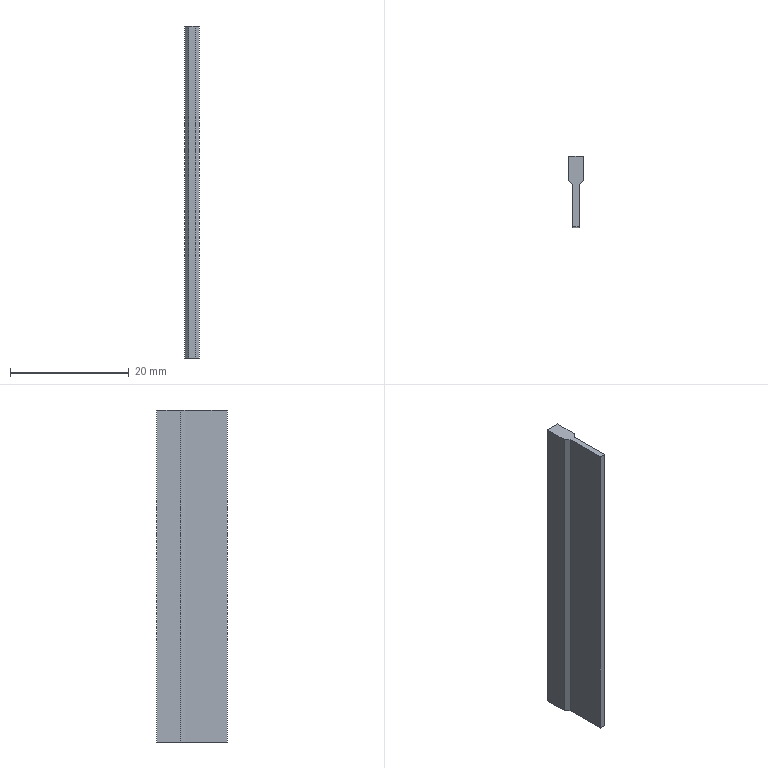Part | NX | features BREP 2 | 2 solids | 20 faces | box 2.42 x 11.896 x 56 mm | volume 2041 mm3 | plane 20
STEP:
#1=CARTESIAN_POINT('',(-0.5101,1.23,-4.));
#2=VERTEX_POINT('',#1);
#3=CARTESIAN_POINT('',(-0.5101,1.23,52.));
#4=VERTEX_POINT('',#3);
#5=CARTESIAN_POINT('',(-0.5101,1.23,0.));
#6=DIRECTION('',(0.,0.,1.));
#7=VECTOR('',#6,1000.);
#8=LINE('',#5,#7);
#9=EDGE_CURVE('',#2,#4,#8,.T.);
#10=ORIENTED_EDGE('',*,*,#9,.T.);
#11=CARTESIAN_POINT('',(-1.21,1.93,52.));
#12=VERTEX_POINT('',#11);
#13=CARTESIAN_POINT('',(-0.5101,1.23,52.));
#14=DIRECTION('',(0.7071,-0.7071,0.));
#15=VECTOR('',#14,1000.);
#16=LINE('',#13,#15);
#17=EDGE_CURVE('',#12,#4,#16,.T.);
#18=ORIENTED_EDGE('',*,*,#17,.F.);
#19=CARTESIAN_POINT('',(-1.21,1.93,-4.));
#20=VERTEX_POINT('',#19);
#21=CARTESIAN_POINT('',(-1.21,1.93,0.));
#22=DIRECTION('',(0.,0.,1.));
#23=VECTOR('',#22,1000.);
#24=LINE('',#21,#23);
#25=EDGE_CURVE('',#20,#12,#24,.T.);
#26=ORIENTED_EDGE('',*,*,#25,.F.);
#27=CARTESIAN_POINT('',(-0.5101,1.23,-4.));
#28=DIRECTION('',(0.7071,-0.7071,0.));
#29=VECTOR('',#28,1000.);
#30=LINE('',#27,#29);
#31=EDGE_CURVE('',#20,#2,#30,.T.);
#32=ORIENTED_EDGE('',*,*,#31,.T.);
#33=EDGE_LOOP('',(#10,#18,#26,#32));
#34=FACE_BOUND('',#33,.T.);
#35=CARTESIAN_POINT('',(-0.5101,1.23,0.));
#36=DIRECTION('',(0.7071,0.7071,0.));
#37=DIRECTION('',(0.7071,-0.7071,0.));
#38=AXIS2_PLACEMENT_3D('',#35,#36,#37);
#39=PLANE('',#38);
#40=ADVANCED_FACE('',(#34),#39,.F.);
#41=ORIENTED_EDGE('',*,*,#25,.T.);
#42=CARTESIAN_POINT('',(-1.21,5.923,52.));
#43=VERTEX_POINT('',#42);
#44=CARTESIAN_POINT('',(-1.21,-19.679,52.));
#45=DIRECTION('',(0.,-1.,0.));
#46=VECTOR('',#45,1000.);
#47=LINE('',#44,#46);
#48=EDGE_CURVE('',#43,#12,#47,.T.);
#49=ORIENTED_EDGE('',*,*,#48,.F.);
#50=CARTESIAN_POINT('',(-1.21,5.923,-4.));
#51=VERTEX_POINT('',#50);
#52=CARTESIAN_POINT('',(-1.21,5.923,0.));
#53=DIRECTION('',(0.,0.,1.));
#54=VECTOR('',#53,1000.);
#55=LINE('',#52,#54);
#56=EDGE_CURVE('',#51,#43,#55,.T.);
#57=ORIENTED_EDGE('',*,*,#56,.F.);
#58=CARTESIAN_POINT('',(-1.21,-19.679,-4.));
#59=DIRECTION('',(0.,-1.,0.));
#60=VECTOR('',#59,1000.);
#61=LINE('',#58,#60);
#62=EDGE_CURVE('',#51,#20,#61,.T.);
#63=ORIENTED_EDGE('',*,*,#62,.T.);
#64=EDGE_LOOP('',(#41,#49,#57,#63));
#65=FACE_BOUND('',#64,.T.);
#66=CARTESIAN_POINT('',(-1.21,1.93,0.));
#67=DIRECTION('',(1.,0.,0.));
#68=DIRECTION('',(0.,-1.,0.));
#69=AXIS2_PLACEMENT_3D('',#66,#67,#68);
#70=PLANE('',#69);
#71=ADVANCED_FACE('',(#65),#70,.F.);
#72=ORIENTED_EDGE('',*,*,#56,.T.);
#73=CARTESIAN_POINT('',(1.21,5.923,52.));
#74=VERTEX_POINT('',#73);
#75=CARTESIAN_POINT('',(-10.54,5.923,52.));
#76=DIRECTION('',(-1.,0.,0.));
#77=VECTOR('',#76,1000.);
#78=LINE('',#75,#77);
#79=EDGE_CURVE('',#74,#43,#78,.T.);
#80=ORIENTED_EDGE('',*,*,#79,.F.);
#81=CARTESIAN_POINT('',(1.21,5.923,-4.));
#82=VERTEX_POINT('',#81);
#83=CARTESIAN_POINT('',(1.21,5.923,0.));
#84=DIRECTION('',(0.,0.,1.));
#85=VECTOR('',#84,1000.);
#86=LINE('',#83,#85);
#87=EDGE_CURVE('',#82,#74,#86,.T.);
#88=ORIENTED_EDGE('',*,*,#87,.F.);
#89=CARTESIAN_POINT('',(-10.54,5.923,-4.));
#90=DIRECTION('',(-1.,0.,0.));
#91=VECTOR('',#90,1000.);
#92=LINE('',#89,#91);
#93=EDGE_CURVE('',#82,#51,#92,.T.);
#94=ORIENTED_EDGE('',*,*,#93,.T.);
#95=EDGE_LOOP('',(#72,#80,#88,#94));
#96=FACE_BOUND('',#95,.T.);
#97=CARTESIAN_POINT('',(-10.54,5.923,0.));
#98=DIRECTION('',(0.,1.,0.));
#99=DIRECTION('',(1.,0.,0.));
#100=AXIS2_PLACEMENT_3D('',#97,#98,#99);
#101=PLANE('',#100);
#102=ADVANCED_FACE('',(#96),#101,.T.);
#103=ORIENTED_EDGE('',*,*,#87,.T.);
#104=CARTESIAN_POINT('',(1.21,1.923,52.));
#105=VERTEX_POINT('',#104);
#106=CARTESIAN_POINT('',(1.21,-19.679,52.));
#107=DIRECTION('',(0.,1.,0.));
#108=VECTOR('',#107,1000.);
#109=LINE('',#106,#108);
#110=EDGE_CURVE('',#105,#74,#109,.T.);
#111=ORIENTED_EDGE('',*,*,#110,.F.);
#112=CARTESIAN_POINT('',(1.21,1.923,-4.));
#113=VERTEX_POINT('',#112);
#114=CARTESIAN_POINT('',(1.21,1.923,0.));
#115=DIRECTION('',(0.,0.,1.));
#116=VECTOR('',#115,1000.);
#117=LINE('',#114,#116);
#118=EDGE_CURVE('',#113,#105,#117,.T.);
#119=ORIENTED_EDGE('',*,*,#118,.F.);
#120=CARTESIAN_POINT('',(1.21,-19.679,-4.));
#121=DIRECTION('',(0.,1.,0.));
#122=VECTOR('',#121,1000.);
#123=LINE('',#120,#122);
#124=EDGE_CURVE('',#113,#82,#123,.T.);
#125=ORIENTED_EDGE('',*,*,#124,.T.);
#126=EDGE_LOOP('',(#103,#111,#119,#125));
#127=FACE_BOUND('',#126,.T.);
#128=CARTESIAN_POINT('',(1.21,5.923,0.));
#129=DIRECTION('',(-1.,0.,0.));
#130=DIRECTION('',(0.,1.,0.));
#131=AXIS2_PLACEMENT_3D('',#128,#129,#130);
#132=PLANE('',#131);
#133=ADVANCED_FACE('',(#127),#132,.F.);
#134=ORIENTED_EDGE('',*,*,#118,.T.);
#135=CARTESIAN_POINT('',(0.5101,1.223,52.));
#136=VERTEX_POINT('',#135);
#137=CARTESIAN_POINT('',(1.21,1.923,52.));
#138=DIRECTION('',(0.7071,0.7071,0.));
#139=VECTOR('',#138,1000.);
#140=LINE('',#137,#139);
#141=EDGE_CURVE('',#136,#105,#140,.T.);
#142=ORIENTED_EDGE('',*,*,#141,.F.);
#143=CARTESIAN_POINT('',(0.5101,1.223,-4.));
#144=VERTEX_POINT('',#143);
#145=CARTESIAN_POINT('',(0.5101,1.223,0.));
#146=DIRECTION('',(0.,0.,1.));
#147=VECTOR('',#146,1000.);
#148=LINE('',#145,#147);
#149=EDGE_CURVE('',#144,#136,#148,.T.);
#150=ORIENTED_EDGE('',*,*,#149,.F.);
#151=CARTESIAN_POINT('',(1.21,1.923,-4.));
#152=DIRECTION('',(0.7071,0.7071,0.));
#153=VECTOR('',#152,1000.);
#154=LINE('',#151,#153);
#155=EDGE_CURVE('',#144,#113,#154,.T.);
#156=ORIENTED_EDGE('',*,*,#155,.T.);
#157=EDGE_LOOP('',(#134,#142,#150,#156));
#158=FACE_BOUND('',#157,.T.);
#159=CARTESIAN_POINT('',(1.21,1.923,0.));
#160=DIRECTION('',(-0.7071,0.7071,0.));
#161=DIRECTION('',(0.7071,0.7071,0.));
#162=AXIS2_PLACEMENT_3D('',#159,#160,#161);
#163=PLANE('',#162);
#164=ADVANCED_FACE('',(#158),#163,.F.);
#165=CARTESIAN_POINT('',(0.5101,-5.973,-4.));
#166=VERTEX_POINT('',#165);
#167=CARTESIAN_POINT('',(0.5101,-5.973,52.));
#168=VERTEX_POINT('',#167);
#169=CARTESIAN_POINT('',(0.5101,-5.973,0.));
#170=DIRECTION('',(0.,0.,1.));
#171=VECTOR('',#170,1000.);
#172=LINE('',#169,#171);
#173=EDGE_CURVE('',#166,#168,#172,.T.);
#174=ORIENTED_EDGE('',*,*,#173,.F.);
#175=CARTESIAN_POINT('',(0.5101,-19.679,-4.));
#176=DIRECTION('',(0.,1.,0.));
#177=VECTOR('',#176,1000.);
#178=LINE('',#175,#177);
#179=EDGE_CURVE('',#166,#144,#178,.T.);
#180=ORIENTED_EDGE('',*,*,#179,.T.);
#181=ORIENTED_EDGE('',*,*,#149,.T.);
#182=CARTESIAN_POINT('',(0.5101,-19.679,52.));
#183=DIRECTION('',(0.,1.,0.));
#184=VECTOR('',#183,1000.);
#185=LINE('',#182,#184);
#186=EDGE_CURVE('',#168,#136,#185,.T.);
#187=ORIENTED_EDGE('',*,*,#186,.F.);
#188=EDGE_LOOP('',(#174,#180,#181,#187));
#189=FACE_BOUND('',#188,.T.);
#190=CARTESIAN_POINT('',(0.5101,-5.28,0.));
#191=DIRECTION('',(-1.,0.,0.));
#192=DIRECTION('',(0.,1.,0.));
#193=AXIS2_PLACEMENT_3D('',#190,#191,#192);
#194=PLANE('',#193);
#195=ADVANCED_FACE('',(#189),#194,.F.);
#196=ORIENTED_EDGE('',*,*,#173,.T.);
#197=CARTESIAN_POINT('',(-0.5101,-5.973,52.));
#198=VERTEX_POINT('',#197);
#199=CARTESIAN_POINT('',(-10.54,-5.973,52.));
#200=DIRECTION('',(1.,0.,0.));
#201=VECTOR('',#200,1000.);
#202=LINE('',#199,#201);
#203=EDGE_CURVE('',#198,#168,#202,.T.);
#204=ORIENTED_EDGE('',*,*,#203,.F.);
#205=CARTESIAN_POINT('',(-0.5101,-5.973,-4.));
#206=VERTEX_POINT('',#205);
#207=CARTESIAN_POINT('',(-0.5101,-5.973,0.));
#208=DIRECTION('',(0.,0.,1.));
#209=VECTOR('',#208,1000.);
#210=LINE('',#207,#209);
#211=EDGE_CURVE('',#206,#198,#210,.T.);
#212=ORIENTED_EDGE('',*,*,#211,.F.);
#213=CARTESIAN_POINT('',(-10.54,-5.973,-4.));
#214=DIRECTION('',(1.,0.,0.));
#215=VECTOR('',#214,1000.);
#216=LINE('',#213,#215);
#217=EDGE_CURVE('',#206,#166,#216,.T.);
#218=ORIENTED_EDGE('',*,*,#217,.T.);
#219=EDGE_LOOP('',(#196,#204,#212,#218));
#220=FACE_BOUND('',#219,.T.);
#221=CARTESIAN_POINT('',(-10.54,-5.973,0.));
#222=DIRECTION('',(0.,-1.,0.));
#223=DIRECTION('',(-1.,0.,0.));
#224=AXIS2_PLACEMENT_3D('',#221,#222,#223);
#225=PLANE('',#224);
#226=ADVANCED_FACE('',(#220),#225,.T.);
#227=CARTESIAN_POINT('',(-0.5101,-19.679,-4.));
#228=DIRECTION('',(0.,-1.,0.));
#229=VECTOR('',#228,1000.);
#230=LINE('',#227,#229);
#231=EDGE_CURVE('',#2,#206,#230,.T.);
#232=ORIENTED_EDGE('',*,*,#231,.T.);
#233=ORIENTED_EDGE('',*,*,#211,.T.);
#234=CARTESIAN_POINT('',(-0.5101,-19.679,52.));
#235=DIRECTION('',(0.,-1.,0.));
#236=VECTOR('',#235,1000.);
#237=LINE('',#234,#236);
#238=EDGE_CURVE('',#4,#198,#237,.T.);
#239=ORIENTED_EDGE('',*,*,#238,.F.);
#240=ORIENTED_EDGE('',*,*,#9,.F.);
#241=EDGE_LOOP('',(#232,#233,#239,#240));
#242=FACE_BOUND('',#241,.T.);
#243=CARTESIAN_POINT('',(-0.5101,-5.28,0.));
#244=DIRECTION('',(1.,0.,0.));
#245=DIRECTION('',(0.,-1.,0.));
#246=AXIS2_PLACEMENT_3D('',#243,#244,#245);
#247=PLANE('',#246);
#248=ADVANCED_FACE('',(#242),#247,.F.);
#249=ORIENTED_EDGE('',*,*,#238,.T.);
#250=ORIENTED_EDGE('',*,*,#203,.T.);
#251=ORIENTED_EDGE('',*,*,#186,.T.);
#252=ORIENTED_EDGE('',*,*,#141,.T.);
#253=ORIENTED_EDGE('',*,*,#110,.T.);
#254=ORIENTED_EDGE('',*,*,#79,.T.);
#255=ORIENTED_EDGE('',*,*,#48,.T.);
#256=ORIENTED_EDGE('',*,*,#17,.T.);
#257=EDGE_LOOP('',(#249,#250,#251,#252,#253,#254,#255,#256));
#258=FACE_BOUND('',#257,.T.);
#259=CARTESIAN_POINT('',(-10.54,-19.679,52.));
#260=DIRECTION('',(0.,0.,1.));
#261=DIRECTION('',(-1.,0.,0.));
#262=AXIS2_PLACEMENT_3D('',#259,#260,#261);
#263=PLANE('',#262);
#264=ADVANCED_FACE('',(#258),#263,.T.);
#265=ORIENTED_EDGE('',*,*,#217,.F.);
#266=ORIENTED_EDGE('',*,*,#231,.F.);
#267=ORIENTED_EDGE('',*,*,#31,.F.);
#268=ORIENTED_EDGE('',*,*,#62,.F.);
#269=ORIENTED_EDGE('',*,*,#93,.F.);
#270=ORIENTED_EDGE('',*,*,#124,.F.);
#271=ORIENTED_EDGE('',*,*,#155,.F.);
#272=ORIENTED_EDGE('',*,*,#179,.F.);
#273=EDGE_LOOP('',(#265,#266,#267,#268,#269,#270,#271,#272));
#274=FACE_BOUND('',#273,.T.);
#275=CARTESIAN_POINT('',(-10.54,-19.679,-4.));
#276=DIRECTION('',(0.,0.,1.));
#277=DIRECTION('',(-1.,0.,0.));
#278=AXIS2_PLACEMENT_3D('',#275,#276,#277);
#279=PLANE('',#278);
#280=ADVANCED_FACE('',(#274),#279,.F.);
#281=CLOSED_SHELL('',(#40,#71,#102,#133,#164,#195,#226,#248,#264,#280));
#282=MANIFOLD_SOLID_BREP('',#281);
#283=CARTESIAN_POINT('',(-0.5101,1.23,-4.));
#284=VERTEX_POINT('',#283);
#285=CARTESIAN_POINT('',(-0.5101,1.23,52.));
#286=VERTEX_POINT('',#285);
#287=CARTESIAN_POINT('',(-0.5101,1.23,0.));
#288=DIRECTION('',(0.,0.,1.));
#289=VECTOR('',#288,1000.);
#290=LINE('',#287,#289);
#291=EDGE_CURVE('',#284,#286,#290,.T.);
#292=ORIENTED_EDGE('',*,*,#291,.T.);
#293=CARTESIAN_POINT('',(-1.21,1.93,52.));
#294=VERTEX_POINT('',#293);
#295=CARTESIAN_POINT('',(-0.5101,1.23,52.));
#296=DIRECTION('',(0.7071,-0.7071,0.));
#297=VECTOR('',#296,1000.);
#298=LINE('',#295,#297);
#299=EDGE_CURVE('',#294,#286,#298,.T.);
#300=ORIENTED_EDGE('',*,*,#299,.F.);
#301=CARTESIAN_POINT('',(-1.21,1.93,-4.));
#302=VERTEX_POINT('',#301);
#303=CARTESIAN_POINT('',(-1.21,1.93,0.));
#304=DIRECTION('',(0.,0.,1.));
#305=VECTOR('',#304,1000.);
#306=LINE('',#303,#305);
#307=EDGE_CURVE('',#302,#294,#306,.T.);
#308=ORIENTED_EDGE('',*,*,#307,.F.);
#309=CARTESIAN_POINT('',(-0.5101,1.23,-4.));
#310=DIRECTION('',(0.7071,-0.7071,0.));
#311=VECTOR('',#310,1000.);
#312=LINE('',#309,#311);
#313=EDGE_CURVE('',#302,#284,#312,.T.);
#314=ORIENTED_EDGE('',*,*,#313,.T.);
#315=EDGE_LOOP('',(#292,#300,#308,#314));
#316=FACE_BOUND('',#315,.T.);
#317=CARTESIAN_POINT('',(-0.5101,1.23,0.));
#318=DIRECTION('',(0.7071,0.7071,0.));
#319=DIRECTION('',(0.7071,-0.7071,0.));
#320=AXIS2_PLACEMENT_3D('',#317,#318,#319);
#321=PLANE('',#320);
#322=ADVANCED_FACE('',(#316),#321,.F.);
#323=ORIENTED_EDGE('',*,*,#307,.T.);
#324=CARTESIAN_POINT('',(-1.21,5.923,52.));
#325=VERTEX_POINT('',#324);
#326=CARTESIAN_POINT('',(-1.21,-19.679,52.));
#327=DIRECTION('',(0.,-1.,0.));
#328=VECTOR('',#327,1000.);
#329=LINE('',#326,#328);
#330=EDGE_CURVE('',#325,#294,#329,.T.);
#331=ORIENTED_EDGE('',*,*,#330,.F.);
#332=CARTESIAN_POINT('',(-1.21,5.923,-4.));
#333=VERTEX_POINT('',#332);
#334=CARTESIAN_POINT('',(-1.21,5.923,0.));
#335=DIRECTION('',(0.,0.,1.));
#336=VECTOR('',#335,1000.);
#337=LINE('',#334,#336);
#338=EDGE_CURVE('',#333,#325,#337,.T.);
#339=ORIENTED_EDGE('',*,*,#338,.F.);
#340=CARTESIAN_POINT('',(-1.21,-19.679,-4.));
#341=DIRECTION('',(0.,-1.,0.));
#342=VECTOR('',#341,1000.);
#343=LINE('',#340,#342);
#344=EDGE_CURVE('',#333,#302,#343,.T.);
#345=ORIENTED_EDGE('',*,*,#344,.T.);
#346=EDGE_LOOP('',(#323,#331,#339,#345));
#347=FACE_BOUND('',#346,.T.);
#348=CARTESIAN_POINT('',(-1.21,1.93,0.));
#349=DIRECTION('',(1.,0.,0.));
#350=DIRECTION('',(0.,-1.,0.));
#351=AXIS2_PLACEMENT_3D('',#348,#349,#350);
#352=PLANE('',#351);
#353=ADVANCED_FACE('',(#347),#352,.F.);
#354=ORIENTED_EDGE('',*,*,#338,.T.);
#355=CARTESIAN_POINT('',(1.21,5.923,52.));
#356=VERTEX_POINT('',#355);
#357=CARTESIAN_POINT('',(-10.54,5.923,52.));
#358=DIRECTION('',(-1.,0.,0.));
#359=VECTOR('',#358,1000.);
#360=LINE('',#357,#359);
#361=EDGE_CURVE('',#356,#325,#360,.T.);
#362=ORIENTED_EDGE('',*,*,#361,.F.);
#363=CARTESIAN_POINT('',(1.21,5.923,-4.));
#364=VERTEX_POINT('',#363);
#365=CARTESIAN_POINT('',(1.21,5.923,0.));
#366=DIRECTION('',(0.,0.,1.));
#367=VECTOR('',#366,1000.);
#368=LINE('',#365,#367);
#369=EDGE_CURVE('',#364,#356,#368,.T.);
#370=ORIENTED_EDGE('',*,*,#369,.F.);
#371=CARTESIAN_POINT('',(-10.54,5.923,-4.));
#372=DIRECTION('',(-1.,0.,0.));
#373=VECTOR('',#372,1000.);
#374=LINE('',#371,#373);
#375=EDGE_CURVE('',#364,#333,#374,.T.);
#376=ORIENTED_EDGE('',*,*,#375,.T.);
#377=EDGE_LOOP('',(#354,#362,#370,#376));
#378=FACE_BOUND('',#377,.T.);
#379=CARTESIAN_POINT('',(-10.54,5.923,0.));
#380=DIRECTION('',(0.,1.,0.));
#381=DIRECTION('',(1.,0.,0.));
#382=AXIS2_PLACEMENT_3D('',#379,#380,#381);
#383=PLANE('',#382);
#384=ADVANCED_FACE('',(#378),#383,.T.);
#385=ORIENTED_EDGE('',*,*,#369,.T.);
#386=CARTESIAN_POINT('',(1.21,1.923,52.));
#387=VERTEX_POINT('',#386);
#388=CARTESIAN_POINT('',(1.21,-19.679,52.));
#389=DIRECTION('',(0.,1.,0.));
#390=VECTOR('',#389,1000.);
#391=LINE('',#388,#390);
#392=EDGE_CURVE('',#387,#356,#391,.T.);
#393=ORIENTED_EDGE('',*,*,#392,.F.);
#394=CARTESIAN_POINT('',(1.21,1.923,-4.));
#395=VERTEX_POINT('',#394);
#396=CARTESIAN_POINT('',(1.21,1.923,0.));
#397=DIRECTION('',(0.,0.,1.));
#398=VECTOR('',#397,1000.);
#399=LINE('',#396,#398);
#400=EDGE_CURVE('',#395,#387,#399,.T.);
#401=ORIENTED_EDGE('',*,*,#400,.F.);
#402=CARTESIAN_POINT('',(1.21,-19.679,-4.));
#403=DIRECTION('',(0.,1.,0.));
#404=VECTOR('',#403,1000.);
#405=LINE('',#402,#404);
#406=EDGE_CURVE('',#395,#364,#405,.T.);
#407=ORIENTED_EDGE('',*,*,#406,.T.);
#408=EDGE_LOOP('',(#385,#393,#401,#407));
#409=FACE_BOUND('',#408,.T.);
#410=CARTESIAN_POINT('',(1.21,5.923,0.));
#411=DIRECTION('',(-1.,0.,0.));
#412=DIRECTION('',(0.,1.,0.));
#413=AXIS2_PLACEMENT_3D('',#410,#411,#412);
#414=PLANE('',#413);
#415=ADVANCED_FACE('',(#409),#414,.F.);
#416=ORIENTED_EDGE('',*,*,#400,.T.);
#417=CARTESIAN_POINT('',(0.5101,1.223,52.));
#418=VERTEX_POINT('',#417);
#419=CARTESIAN_POINT('',(1.21,1.923,52.));
#420=DIRECTION('',(0.7071,0.7071,0.));
#421=VECTOR('',#420,1000.);
#422=LINE('',#419,#421);
#423=EDGE_CURVE('',#418,#387,#422,.T.);
#424=ORIENTED_EDGE('',*,*,#423,.F.);
#425=CARTESIAN_POINT('',(0.5101,1.223,-4.));
#426=VERTEX_POINT('',#425);
#427=CARTESIAN_POINT('',(0.5101,1.223,0.));
#428=DIRECTION('',(0.,0.,1.));
#429=VECTOR('',#428,1000.);
#430=LINE('',#427,#429);
#431=EDGE_CURVE('',#426,#418,#430,.T.);
#432=ORIENTED_EDGE('',*,*,#431,.F.);
#433=CARTESIAN_POINT('',(1.21,1.923,-4.));
#434=DIRECTION('',(0.7071,0.7071,0.));
#435=VECTOR('',#434,1000.);
#436=LINE('',#433,#435);
#437=EDGE_CURVE('',#426,#395,#436,.T.);
#438=ORIENTED_EDGE('',*,*,#437,.T.);
#439=EDGE_LOOP('',(#416,#424,#432,#438));
#440=FACE_BOUND('',#439,.T.);
#441=CARTESIAN_POINT('',(1.21,1.923,0.));
#442=DIRECTION('',(-0.7071,0.7071,0.));
#443=DIRECTION('',(0.7071,0.7071,0.));
#444=AXIS2_PLACEMENT_3D('',#441,#442,#443);
#445=PLANE('',#444);
#446=ADVANCED_FACE('',(#440),#445,.F.);
#447=CARTESIAN_POINT('',(0.5101,-5.973,-4.));
#448=VERTEX_POINT('',#447);
#449=CARTESIAN_POINT('',(0.5101,-5.973,52.));
#450=VERTEX_POINT('',#449);
#451=CARTESIAN_POINT('',(0.5101,-5.973,0.));
#452=DIRECTION('',(0.,0.,1.));
#453=VECTOR('',#452,1000.);
#454=LINE('',#451,#453);
#455=EDGE_CURVE('',#448,#450,#454,.T.);
#456=ORIENTED_EDGE('',*,*,#455,.F.);
#457=CARTESIAN_POINT('',(0.5101,-19.679,-4.));
#458=DIRECTION('',(0.,1.,0.));
#459=VECTOR('',#458,1000.);
#460=LINE('',#457,#459);
#461=EDGE_CURVE('',#448,#426,#460,.T.);
#462=ORIENTED_EDGE('',*,*,#461,.T.);
#463=ORIENTED_EDGE('',*,*,#431,.T.);
#464=CARTESIAN_POINT('',(0.5101,-19.679,52.));
#465=DIRECTION('',(0.,1.,0.));
#466=VECTOR('',#465,1000.);
#467=LINE('',#464,#466);
#468=EDGE_CURVE('',#450,#418,#467,.T.);
#469=ORIENTED_EDGE('',*,*,#468,.F.);
#470=EDGE_LOOP('',(#456,#462,#463,#469));
#471=FACE_BOUND('',#470,.T.);
#472=CARTESIAN_POINT('',(0.5101,-5.28,0.));
#473=DIRECTION('',(-1.,0.,0.));
#474=DIRECTION('',(0.,1.,0.));
#475=AXIS2_PLACEMENT_3D('',#472,#473,#474);
#476=PLANE('',#475);
#477=ADVANCED_FACE('',(#471),#476,.F.);
#478=ORIENTED_EDGE('',*,*,#455,.T.);
#479=CARTESIAN_POINT('',(-0.5101,-5.973,52.));
#480=VERTEX_POINT('',#479);
#481=CARTESIAN_POINT('',(-10.54,-5.973,52.));
#482=DIRECTION('',(1.,0.,0.));
#483=VECTOR('',#482,1000.);
#484=LINE('',#481,#483);
#485=EDGE_CURVE('',#480,#450,#484,.T.);
#486=ORIENTED_EDGE('',*,*,#485,.F.);
#487=CARTESIAN_POINT('',(-0.5101,-5.973,-4.));
#488=VERTEX_POINT('',#487);
#489=CARTESIAN_POINT('',(-0.5101,-5.973,0.));
#490=DIRECTION('',(0.,0.,1.));
#491=VECTOR('',#490,1000.);
#492=LINE('',#489,#491);
#493=EDGE_CURVE('',#488,#480,#492,.T.);
#494=ORIENTED_EDGE('',*,*,#493,.F.);
#495=CARTESIAN_POINT('',(-10.54,-5.973,-4.));
#496=DIRECTION('',(1.,0.,0.));
#497=VECTOR('',#496,1000.);
#498=LINE('',#495,#497);
#499=EDGE_CURVE('',#488,#448,#498,.T.);
#500=ORIENTED_EDGE('',*,*,#499,.T.);
#501=EDGE_LOOP('',(#478,#486,#494,#500));
#502=FACE_BOUND('',#501,.T.);
#503=CARTESIAN_POINT('',(-10.54,-5.973,0.));
#504=DIRECTION('',(0.,-1.,0.));
#505=DIRECTION('',(-1.,0.,0.));
#506=AXIS2_PLACEMENT_3D('',#503,#504,#505);
#507=PLANE('',#506);
#508=ADVANCED_FACE('',(#502),#507,.T.);
#509=CARTESIAN_POINT('',(-0.5101,-19.679,-4.));
#510=DIRECTION('',(0.,-1.,0.));
#511=VECTOR('',#510,1000.);
#512=LINE('',#509,#511);
#513=EDGE_CURVE('',#284,#488,#512,.T.);
#514=ORIENTED_EDGE('',*,*,#513,.T.);
#515=ORIENTED_EDGE('',*,*,#493,.T.);
#516=CARTESIAN_POINT('',(-0.5101,-19.679,52.));
#517=DIRECTION('',(0.,-1.,0.));
#518=VECTOR('',#517,1000.);
#519=LINE('',#516,#518);
#520=EDGE_CURVE('',#286,#480,#519,.T.);
#521=ORIENTED_EDGE('',*,*,#520,.F.);
#522=ORIENTED_EDGE('',*,*,#291,.F.);
#523=EDGE_LOOP('',(#514,#515,#521,#522));
#524=FACE_BOUND('',#523,.T.);
#525=CARTESIAN_POINT('',(-0.5101,-5.28,0.));
#526=DIRECTION('',(1.,0.,0.));
#527=DIRECTION('',(0.,-1.,0.));
#528=AXIS2_PLACEMENT_3D('',#525,#526,#527);
#529=PLANE('',#528);
#530=ADVANCED_FACE('',(#524),#529,.F.);
#531=ORIENTED_EDGE('',*,*,#520,.T.);
#532=ORIENTED_EDGE('',*,*,#485,.T.);
#533=ORIENTED_EDGE('',*,*,#468,.T.);
#534=ORIENTED_EDGE('',*,*,#423,.T.);
#535=ORIENTED_EDGE('',*,*,#392,.T.);
#536=ORIENTED_EDGE('',*,*,#361,.T.);
#537=ORIENTED_EDGE('',*,*,#330,.T.);
#538=ORIENTED_EDGE('',*,*,#299,.T.);
#539=EDGE_LOOP('',(#531,#532,#533,#534,#535,#536,#537,#538));
#540=FACE_BOUND('',#539,.T.);
#541=CARTESIAN_POINT('',(-10.54,-19.679,52.));
#542=DIRECTION('',(0.,0.,1.));
#543=DIRECTION('',(-1.,0.,0.));
#544=AXIS2_PLACEMENT_3D('',#541,#542,#543);
#545=PLANE('',#544);
#546=ADVANCED_FACE('',(#540),#545,.T.);
#547=ORIENTED_EDGE('',*,*,#499,.F.);
#548=ORIENTED_EDGE('',*,*,#513,.F.);
#549=ORIENTED_EDGE('',*,*,#313,.F.);
#550=ORIENTED_EDGE('',*,*,#344,.F.);
#551=ORIENTED_EDGE('',*,*,#375,.F.);
#552=ORIENTED_EDGE('',*,*,#406,.F.);
#553=ORIENTED_EDGE('',*,*,#437,.F.);
#554=ORIENTED_EDGE('',*,*,#461,.F.);
#555=EDGE_LOOP('',(#547,#548,#549,#550,#551,#552,#553,#554));
#556=FACE_BOUND('',#555,.T.);
#557=CARTESIAN_POINT('',(-10.54,-19.679,-4.));
#558=DIRECTION('',(0.,0.,1.));
#559=DIRECTION('',(-1.,0.,0.));
#560=AXIS2_PLACEMENT_3D('',#557,#558,#559);
#561=PLANE('',#560);
#562=ADVANCED_FACE('',(#556),#561,.F.);
#563=CLOSED_SHELL('',(#322,#353,#384,#415,#446,#477,#508,#530,#546,#562));
#564=MANIFOLD_SOLID_BREP('',#563);
#565=(LENGTH_UNIT()NAMED_UNIT(*)SI_UNIT(.MILLI.,.METRE.));
#566=UNCERTAINTY_MEASURE_WITH_UNIT(LENGTH_MEASURE(0.00001),#565,'','');
#567=(NAMED_UNIT(*)PLANE_ANGLE_UNIT()SI_UNIT($,.RADIAN.));
#568=(NAMED_UNIT(*)SI_UNIT($,.STERADIAN.)SOLID_ANGLE_UNIT());
#569=(GEOMETRIC_REPRESENTATION_CONTEXT(3)GLOBAL_UNCERTAINTY_ASSIGNED_CONTEXT((#566))GLOBAL_UNIT_ASSIGNED_CONTEXT((#565,#567,#568))REPRESENTATION_CONTEXT('',''));
#570=ADVANCED_BREP_SHAPE_REPRESENTATION('',(#282,#564),#569);